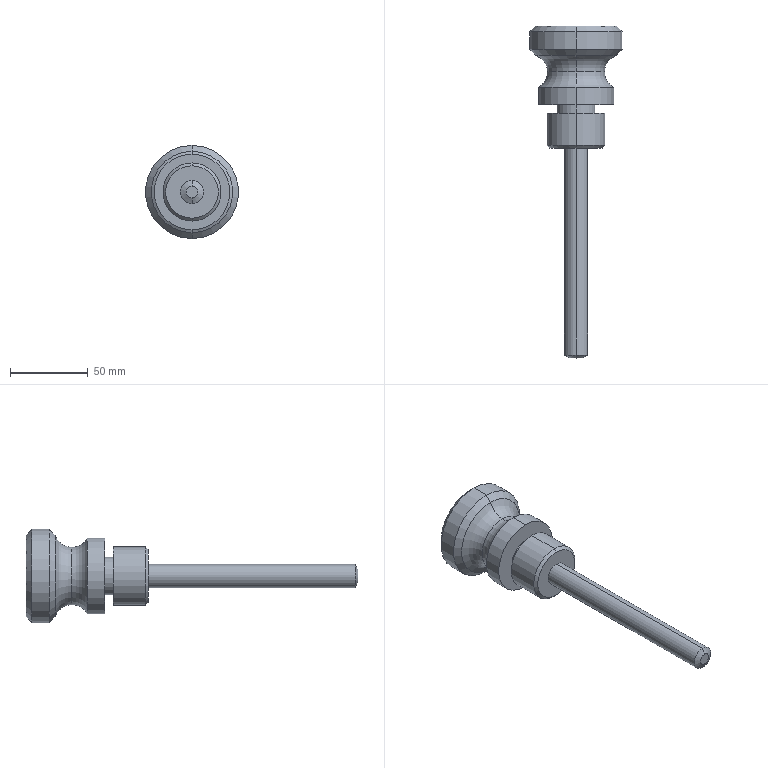Part | SolidWorks | features Revolution 1, Scale 1 | 1 solid | 27 faces | box 60 x 213.75 x 60 mm | volume 149521 mm3 | cylinder 10 | cone 8 | plane 5 | torus 4 | commonest cylinder face diameters 15 x2 24.375 x2 37.5 x2 48.75 x2 60 x2
STEP:
#1=CARTESIAN_POINT('',(0.,6.534,26.25));
#2=VERTEX_POINT('',#1);
#3=CARTESIAN_POINT('',(0.,-4.176,18.442));
#4=VERTEX_POINT('',#3);
#5=CARTESIAN_POINT('',(0.,-4.176,29.692));
#6=DIRECTION('',(-1.,0.,0.));
#7=DIRECTION('',(0.,0.,1.));
#8=AXIS2_PLACEMENT_3D('',#5,#6,#7);
#9=CIRCLE('',#8,11.25);
#10=EDGE_CURVE('',#2,#4,#9,.T.);
#11=ORIENTED_EDGE('',*,*,#10,.T.);
#12=CARTESIAN_POINT('',(0.,-4.176,-18.442));
#13=VERTEX_POINT('',#12);
#14=CARTESIAN_POINT('',(0.,-4.176,0.));
#15=DIRECTION('',(0.,1.,0.));
#16=DIRECTION('',(0.,0.,1.));
#17=AXIS2_PLACEMENT_3D('',#14,#15,#16);
#18=CIRCLE('',#17,18.442);
#19=EDGE_CURVE('',#4,#13,#18,.T.);
#20=ORIENTED_EDGE('',*,*,#19,.T.);
#21=CARTESIAN_POINT('',(0.,6.534,-26.25));
#22=VERTEX_POINT('',#21);
#23=CARTESIAN_POINT('',(0.,-4.176,-29.692));
#24=DIRECTION('',(1.,0.,0.));
#25=DIRECTION('',(0.,0.,-1.));
#26=AXIS2_PLACEMENT_3D('',#23,#24,#25);
#27=CIRCLE('',#26,11.25);
#28=EDGE_CURVE('',#22,#13,#27,.T.);
#29=ORIENTED_EDGE('',*,*,#28,.F.);
#30=CARTESIAN_POINT('',(0.,6.534,0.));
#31=DIRECTION('',(0.,1.,0.));
#32=DIRECTION('',(0.,0.,1.));
#33=AXIS2_PLACEMENT_3D('',#30,#31,#32);
#34=CIRCLE('',#33,26.25);
#35=EDGE_CURVE('',#2,#22,#34,.T.);
#36=ORIENTED_EDGE('',*,*,#35,.F.);
#37=EDGE_LOOP('',(#11,#20,#29,#36));
#38=FACE_OUTER_BOUND('',#37,.T.);
#39=CARTESIAN_POINT('',(0.,-4.176,0.));
#40=DIRECTION('',(0.,1.,0.));
#41=DIRECTION('',(0.,0.,1.));
#42=AXIS2_PLACEMENT_3D('',#39,#40,#41);
#43=TOROIDAL_SURFACE('',#42,29.692,11.25);
#44=ADVANCED_FACE('',(#38),#43,.F.);
#45=ORIENTED_EDGE('',*,*,#28,.T.);
#46=CARTESIAN_POINT('',(0.,-4.176,0.));
#47=DIRECTION('',(0.,1.,0.));
#48=DIRECTION('',(0.,0.,1.));
#49=AXIS2_PLACEMENT_3D('',#46,#47,#48);
#50=CIRCLE('',#49,18.442);
#51=EDGE_CURVE('',#13,#4,#50,.T.);
#52=ORIENTED_EDGE('',*,*,#51,.T.);
#53=ORIENTED_EDGE('',*,*,#10,.F.);
#54=CARTESIAN_POINT('',(0.,6.534,0.));
#55=DIRECTION('',(0.,1.,0.));
#56=DIRECTION('',(0.,0.,1.));
#57=AXIS2_PLACEMENT_3D('',#54,#55,#56);
#58=CIRCLE('',#57,26.25);
#59=EDGE_CURVE('',#22,#2,#58,.T.);
#60=ORIENTED_EDGE('',*,*,#59,.F.);
#61=EDGE_LOOP('',(#45,#52,#53,#60));
#62=FACE_OUTER_BOUND('',#61,.T.);
#63=CARTESIAN_POINT('',(0.,-4.176,0.));
#64=DIRECTION('',(0.,1.,0.));
#65=DIRECTION('',(0.,0.,1.));
#66=AXIS2_PLACEMENT_3D('',#63,#64,#65);
#67=TOROIDAL_SURFACE('',#66,29.692,11.25);
#68=ADVANCED_FACE('',(#62),#67,.F.);
#69=CARTESIAN_POINT('',(0.,-186.591,7.5));
#70=VERTEX_POINT('',#69);
#71=CARTESIAN_POINT('',(0.,-186.591,-7.5));
#72=VERTEX_POINT('',#71);
#73=CARTESIAN_POINT('',(0.,-186.591,0.));
#74=DIRECTION('',(0.,1.,0.));
#75=DIRECTION('',(0.,0.,1.));
#76=AXIS2_PLACEMENT_3D('',#73,#74,#75);
#77=CIRCLE('',#76,7.5);
#78=EDGE_CURVE('',#70,#72,#77,.T.);
#79=ORIENTED_EDGE('',*,*,#78,.T.);
#80=CARTESIAN_POINT('',(0.,-53.466,-7.5));
#81=VERTEX_POINT('',#80);
#82=CARTESIAN_POINT('',(0.,25.284,-7.5));
#83=DIRECTION('',(0.,1.,0.));
#84=VECTOR('',#83,1000.);
#85=LINE('',#82,#84);
#86=EDGE_CURVE('',#72,#81,#85,.T.);
#87=ORIENTED_EDGE('',*,*,#86,.T.);
#88=CARTESIAN_POINT('',(0.,-53.466,7.5));
#89=VERTEX_POINT('',#88);
#90=CARTESIAN_POINT('',(0.,-53.466,0.));
#91=DIRECTION('',(0.,1.,0.));
#92=DIRECTION('',(0.,0.,1.));
#93=AXIS2_PLACEMENT_3D('',#90,#91,#92);
#94=CIRCLE('',#93,7.5);
#95=EDGE_CURVE('',#89,#81,#94,.T.);
#96=ORIENTED_EDGE('',*,*,#95,.F.);
#97=CARTESIAN_POINT('',(0.,25.284,7.5));
#98=DIRECTION('',(0.,1.,0.));
#99=VECTOR('',#98,1000.);
#100=LINE('',#97,#99);
#101=EDGE_CURVE('',#70,#89,#100,.T.);
#102=ORIENTED_EDGE('',*,*,#101,.F.);
#103=EDGE_LOOP('',(#79,#87,#96,#102));
#104=FACE_OUTER_BOUND('',#103,.T.);
#105=CARTESIAN_POINT('',(0.,25.284,0.));
#106=DIRECTION('',(0.,1.,0.));
#107=DIRECTION('',(0.,0.,1.));
#108=AXIS2_PLACEMENT_3D('',#105,#106,#107);
#109=CYLINDRICAL_SURFACE('',#108,7.5);
#110=ADVANCED_FACE('',(#104),#109,.T.);
#111=CARTESIAN_POINT('',(0.,-188.466,3.75));
#112=VERTEX_POINT('',#111);
#113=CARTESIAN_POINT('',(0.,-188.466,-3.75));
#114=VERTEX_POINT('',#113);
#115=CARTESIAN_POINT('',(0.,-188.466,0.));
#116=DIRECTION('',(0.,1.,0.));
#117=DIRECTION('',(0.,0.,1.));
#118=AXIS2_PLACEMENT_3D('',#115,#116,#117);
#119=CIRCLE('',#118,3.75);
#120=EDGE_CURVE('',#112,#114,#119,.T.);
#121=ORIENTED_EDGE('',*,*,#120,.T.);
#122=CARTESIAN_POINT('',(0.,-188.466,-3.75));
#123=DIRECTION('',(0.,0.4472,-0.8944));
#124=VECTOR('',#123,1000.);
#125=LINE('',#122,#124);
#126=EDGE_CURVE('',#114,#72,#125,.T.);
#127=ORIENTED_EDGE('',*,*,#126,.T.);
#128=ORIENTED_EDGE('',*,*,#78,.F.);
#129=CARTESIAN_POINT('',(0.,-188.466,3.75));
#130=DIRECTION('',(0.,0.4472,0.8944));
#131=VECTOR('',#130,1000.);
#132=LINE('',#129,#131);
#133=EDGE_CURVE('',#112,#70,#132,.T.);
#134=ORIENTED_EDGE('',*,*,#133,.F.);
#135=EDGE_LOOP('',(#121,#127,#128,#134));
#136=FACE_OUTER_BOUND('',#135,.T.);
#137=CARTESIAN_POINT('',(0.,-188.466,0.));
#138=DIRECTION('',(0.,1.,0.));
#139=DIRECTION('',(0.,0.,1.));
#140=AXIS2_PLACEMENT_3D('',#137,#138,#139);
#141=CONICAL_SURFACE('',#140,3.75,1.107);
#142=ADVANCED_FACE('',(#136),#141,.T.);
#143=CARTESIAN_POINT('',(0.,25.284,26.25));
#144=VERTEX_POINT('',#143);
#145=CARTESIAN_POINT('',(0.,25.284,-26.25));
#146=VERTEX_POINT('',#145);
#147=CARTESIAN_POINT('',(0.,25.284,0.));
#148=DIRECTION('',(0.,1.,0.));
#149=DIRECTION('',(0.,0.,1.));
#150=AXIS2_PLACEMENT_3D('',#147,#148,#149);
#151=CIRCLE('',#150,26.25);
#152=EDGE_CURVE('',#144,#146,#151,.T.);
#153=ORIENTED_EDGE('',*,*,#152,.F.);
#154=CARTESIAN_POINT('',(0.,21.534,30.));
#155=VERTEX_POINT('',#154);
#156=CARTESIAN_POINT('',(0.,21.534,30.));
#157=DIRECTION('',(0.,-0.7071,0.7071));
#158=VECTOR('',#157,1000.);
#159=LINE('',#156,#158);
#160=EDGE_CURVE('',#144,#155,#159,.T.);
#161=ORIENTED_EDGE('',*,*,#160,.T.);
#162=CARTESIAN_POINT('',(0.,21.534,-30.));
#163=VERTEX_POINT('',#162);
#164=CARTESIAN_POINT('',(0.,21.534,0.));
#165=DIRECTION('',(0.,1.,0.));
#166=DIRECTION('',(0.,0.,1.));
#167=AXIS2_PLACEMENT_3D('',#164,#165,#166);
#168=CIRCLE('',#167,30.);
#169=EDGE_CURVE('',#155,#163,#168,.T.);
#170=ORIENTED_EDGE('',*,*,#169,.T.);
#171=CARTESIAN_POINT('',(0.,21.534,-30.));
#172=DIRECTION('',(0.,-0.7071,-0.7071));
#173=VECTOR('',#172,1000.);
#174=LINE('',#171,#173);
#175=EDGE_CURVE('',#146,#163,#174,.T.);
#176=ORIENTED_EDGE('',*,*,#175,.F.);
#177=EDGE_LOOP('',(#153,#161,#170,#176));
#178=FACE_OUTER_BOUND('',#177,.T.);
#179=CARTESIAN_POINT('',(0.,21.534,0.));
#180=DIRECTION('',(0.,-1.,0.));
#181=DIRECTION('',(0.,0.,-1.));
#182=AXIS2_PLACEMENT_3D('',#179,#180,#181);
#183=CONICAL_SURFACE('',#182,30.,0.7854);
#184=ADVANCED_FACE('',(#178),#183,.T.);
#185=CARTESIAN_POINT('',(0.,10.284,30.));
#186=VERTEX_POINT('',#185);
#187=CARTESIAN_POINT('',(0.,10.284,-30.));
#188=VERTEX_POINT('',#187);
#189=CARTESIAN_POINT('',(0.,10.284,0.));
#190=DIRECTION('',(0.,1.,0.));
#191=DIRECTION('',(0.,0.,1.));
#192=AXIS2_PLACEMENT_3D('',#189,#190,#191);
#193=CIRCLE('',#192,30.);
#194=EDGE_CURVE('',#186,#188,#193,.T.);
#195=ORIENTED_EDGE('',*,*,#194,.T.);
#196=CARTESIAN_POINT('',(0.,25.284,-30.));
#197=DIRECTION('',(0.,1.,0.));
#198=VECTOR('',#197,1000.);
#199=LINE('',#196,#198);
#200=EDGE_CURVE('',#188,#163,#199,.T.);
#201=ORIENTED_EDGE('',*,*,#200,.T.);
#202=ORIENTED_EDGE('',*,*,#169,.F.);
#203=CARTESIAN_POINT('',(0.,25.284,30.));
#204=DIRECTION('',(0.,1.,0.));
#205=VECTOR('',#204,1000.);
#206=LINE('',#203,#205);
#207=EDGE_CURVE('',#186,#155,#206,.T.);
#208=ORIENTED_EDGE('',*,*,#207,.F.);
#209=EDGE_LOOP('',(#195,#201,#202,#208));
#210=FACE_OUTER_BOUND('',#209,.T.);
#211=CARTESIAN_POINT('',(0.,25.284,0.));
#212=DIRECTION('',(0.,1.,0.));
#213=DIRECTION('',(0.,0.,1.));
#214=AXIS2_PLACEMENT_3D('',#211,#212,#213);
#215=CYLINDRICAL_SURFACE('',#214,30.);
#216=ADVANCED_FACE('',(#210),#215,.T.);
#217=ORIENTED_EDGE('',*,*,#35,.T.);
#218=CARTESIAN_POINT('',(0.,6.534,-26.25));
#219=DIRECTION('',(0.,0.7071,-0.7071));
#220=VECTOR('',#219,1000.);
#221=LINE('',#218,#220);
#222=EDGE_CURVE('',#22,#188,#221,.T.);
#223=ORIENTED_EDGE('',*,*,#222,.T.);
#224=ORIENTED_EDGE('',*,*,#194,.F.);
#225=CARTESIAN_POINT('',(0.,6.534,26.25));
#226=DIRECTION('',(0.,0.7071,0.7071));
#227=VECTOR('',#226,1000.);
#228=LINE('',#225,#227);
#229=EDGE_CURVE('',#2,#186,#228,.T.);
#230=ORIENTED_EDGE('',*,*,#229,.F.);
#231=EDGE_LOOP('',(#217,#223,#224,#230));
#232=FACE_OUTER_BOUND('',#231,.T.);
#233=CARTESIAN_POINT('',(0.,6.534,0.));
#234=DIRECTION('',(0.,1.,0.));
#235=DIRECTION('',(0.,0.,1.));
#236=AXIS2_PLACEMENT_3D('',#233,#234,#235);
#237=CONICAL_SURFACE('',#236,26.25,0.7854);
#238=ADVANCED_FACE('',(#232),#237,.T.);
#239=ORIENTED_EDGE('',*,*,#51,.F.);
#240=CARTESIAN_POINT('',(0.,-14.091,-24.375));
#241=VERTEX_POINT('',#240);
#242=CARTESIAN_POINT('',(0.,-4.176,-29.692));
#243=DIRECTION('',(1.,0.,0.));
#244=DIRECTION('',(0.,0.,-1.));
#245=AXIS2_PLACEMENT_3D('',#242,#243,#244);
#246=CIRCLE('',#245,11.25);
#247=EDGE_CURVE('',#13,#241,#246,.T.);
#248=ORIENTED_EDGE('',*,*,#247,.T.);
#249=CARTESIAN_POINT('',(0.,-14.091,24.375));
#250=VERTEX_POINT('',#249);
#251=CARTESIAN_POINT('',(0.,-14.091,0.));
#252=DIRECTION('',(0.,1.,0.));
#253=DIRECTION('',(0.,0.,1.));
#254=AXIS2_PLACEMENT_3D('',#251,#252,#253);
#255=CIRCLE('',#254,24.375);
#256=EDGE_CURVE('',#241,#250,#255,.T.);
#257=ORIENTED_EDGE('',*,*,#256,.T.);
#258=CARTESIAN_POINT('',(0.,-4.176,29.692));
#259=DIRECTION('',(-1.,0.,0.));
#260=DIRECTION('',(0.,0.,1.));
#261=AXIS2_PLACEMENT_3D('',#258,#259,#260);
#262=CIRCLE('',#261,11.25);
#263=EDGE_CURVE('',#4,#250,#262,.T.);
#264=ORIENTED_EDGE('',*,*,#263,.F.);
#265=EDGE_LOOP('',(#239,#248,#257,#264));
#266=FACE_OUTER_BOUND('',#265,.T.);
#267=CARTESIAN_POINT('',(0.,-4.176,0.));
#268=DIRECTION('',(0.,1.,0.));
#269=DIRECTION('',(0.,0.,1.));
#270=AXIS2_PLACEMENT_3D('',#267,#268,#269);
#271=TOROIDAL_SURFACE('',#270,29.692,11.25);
#272=ADVANCED_FACE('',(#266),#271,.F.);
#273=CARTESIAN_POINT('',(0.,-25.341,24.375));
#274=VERTEX_POINT('',#273);
#275=CARTESIAN_POINT('',(0.,-25.341,-24.375));
#276=VERTEX_POINT('',#275);
#277=CARTESIAN_POINT('',(0.,-25.341,0.));
#278=DIRECTION('',(0.,1.,0.));
#279=DIRECTION('',(0.,0.,1.));
#280=AXIS2_PLACEMENT_3D('',#277,#278,#279);
#281=CIRCLE('',#280,24.375);
#282=EDGE_CURVE('',#274,#276,#281,.T.);
#283=ORIENTED_EDGE('',*,*,#282,.T.);
#284=CARTESIAN_POINT('',(0.,25.284,-24.375));
#285=DIRECTION('',(0.,1.,0.));
#286=VECTOR('',#285,1000.);
#287=LINE('',#284,#286);
#288=EDGE_CURVE('',#276,#241,#287,.T.);
#289=ORIENTED_EDGE('',*,*,#288,.T.);
#290=CARTESIAN_POINT('',(0.,-14.091,0.));
#291=DIRECTION('',(0.,1.,0.));
#292=DIRECTION('',(0.,0.,1.));
#293=AXIS2_PLACEMENT_3D('',#290,#291,#292);
#294=CIRCLE('',#293,24.375);
#295=EDGE_CURVE('',#250,#241,#294,.T.);
#296=ORIENTED_EDGE('',*,*,#295,.F.);
#297=CARTESIAN_POINT('',(0.,25.284,24.375));
#298=DIRECTION('',(0.,1.,0.));
#299=VECTOR('',#298,1000.);
#300=LINE('',#297,#299);
#301=EDGE_CURVE('',#274,#250,#300,.T.);
#302=ORIENTED_EDGE('',*,*,#301,.F.);
#303=EDGE_LOOP('',(#283,#289,#296,#302));
#304=FACE_OUTER_BOUND('',#303,.T.);
#305=CARTESIAN_POINT('',(0.,25.284,0.));
#306=DIRECTION('',(0.,1.,0.));
#307=DIRECTION('',(0.,0.,1.));
#308=AXIS2_PLACEMENT_3D('',#305,#306,#307);
#309=CYLINDRICAL_SURFACE('',#308,24.375);
#310=ADVANCED_FACE('',(#304),#309,.T.);
#311=CARTESIAN_POINT('',(0.,-30.966,12.187));
#312=VERTEX_POINT('',#311);
#313=CARTESIAN_POINT('',(0.,-30.966,-12.188));
#314=VERTEX_POINT('',#313);
#315=CARTESIAN_POINT('',(0.,-30.966,0.));
#316=DIRECTION('',(0.,1.,0.));
#317=DIRECTION('',(0.,0.,1.));
#318=AXIS2_PLACEMENT_3D('',#315,#316,#317);
#319=CIRCLE('',#318,12.187);
#320=EDGE_CURVE('',#312,#314,#319,.T.);
#321=ORIENTED_EDGE('',*,*,#320,.T.);
#322=CARTESIAN_POINT('',(0.,-25.341,-12.187));
#323=VERTEX_POINT('',#322);
#324=CARTESIAN_POINT('',(0.,25.284,-12.187));
#325=DIRECTION('',(0.,1.,0.));
#326=VECTOR('',#325,1000.);
#327=LINE('',#324,#326);
#328=EDGE_CURVE('',#314,#323,#327,.T.);
#329=ORIENTED_EDGE('',*,*,#328,.T.);
#330=CARTESIAN_POINT('',(0.,-25.341,12.187));
#331=VERTEX_POINT('',#330);
#332=CARTESIAN_POINT('',(0.,-25.341,0.));
#333=DIRECTION('',(0.,1.,0.));
#334=DIRECTION('',(0.,0.,1.));
#335=AXIS2_PLACEMENT_3D('',#332,#333,#334);
#336=CIRCLE('',#335,12.187);
#337=EDGE_CURVE('',#331,#323,#336,.T.);
#338=ORIENTED_EDGE('',*,*,#337,.F.);
#339=CARTESIAN_POINT('',(0.,25.284,12.187));
#340=DIRECTION('',(0.,1.,0.));
#341=VECTOR('',#340,1000.);
#342=LINE('',#339,#341);
#343=EDGE_CURVE('',#312,#331,#342,.T.);
#344=ORIENTED_EDGE('',*,*,#343,.F.);
#345=EDGE_LOOP('',(#321,#329,#338,#344));
#346=FACE_OUTER_BOUND('',#345,.T.);
#347=CARTESIAN_POINT('',(0.,25.284,0.));
#348=DIRECTION('',(0.,1.,0.));
#349=DIRECTION('',(0.,0.,1.));
#350=AXIS2_PLACEMENT_3D('',#347,#348,#349);
#351=CYLINDRICAL_SURFACE('',#350,12.187);
#352=ADVANCED_FACE('',(#346),#351,.T.);
#353=CARTESIAN_POINT('',(0.,-51.591,18.75));
#354=VERTEX_POINT('',#353);
#355=CARTESIAN_POINT('',(0.,-51.591,-18.75));
#356=VERTEX_POINT('',#355);
#357=CARTESIAN_POINT('',(0.,-51.591,0.));
#358=DIRECTION('',(0.,1.,0.));
#359=DIRECTION('',(0.,0.,1.));
#360=AXIS2_PLACEMENT_3D('',#357,#358,#359);
#361=CIRCLE('',#360,18.75);
#362=EDGE_CURVE('',#354,#356,#361,.T.);
#363=ORIENTED_EDGE('',*,*,#362,.T.);
#364=CARTESIAN_POINT('',(0.,-30.966,-18.75));
#365=VERTEX_POINT('',#364);
#366=CARTESIAN_POINT('',(0.,25.284,-18.75));
#367=DIRECTION('',(0.,1.,0.));
#368=VECTOR('',#367,1000.);
#369=LINE('',#366,#368);
#370=EDGE_CURVE('',#356,#365,#369,.T.);
#371=ORIENTED_EDGE('',*,*,#370,.T.);
#372=CARTESIAN_POINT('',(0.,-30.966,18.75));
#373=VERTEX_POINT('',#372);
#374=CARTESIAN_POINT('',(0.,-30.966,0.));
#375=DIRECTION('',(0.,1.,0.));
#376=DIRECTION('',(0.,0.,1.));
#377=AXIS2_PLACEMENT_3D('',#374,#375,#376);
#378=CIRCLE('',#377,18.75);
#379=EDGE_CURVE('',#373,#365,#378,.T.);
#380=ORIENTED_EDGE('',*,*,#379,.F.);
#381=CARTESIAN_POINT('',(0.,25.284,18.75));
#382=DIRECTION('',(0.,1.,0.));
#383=VECTOR('',#382,1000.);
#384=LINE('',#381,#383);
#385=EDGE_CURVE('',#354,#373,#384,.T.);
#386=ORIENTED_EDGE('',*,*,#385,.F.);
#387=EDGE_LOOP('',(#363,#371,#380,#386));
#388=FACE_OUTER_BOUND('',#387,.T.);
#389=CARTESIAN_POINT('',(0.,25.284,0.));
#390=DIRECTION('',(0.,1.,0.));
#391=DIRECTION('',(0.,0.,1.));
#392=AXIS2_PLACEMENT_3D('',#389,#390,#391);
#393=CYLINDRICAL_SURFACE('',#392,18.75);
#394=ADVANCED_FACE('',(#388),#393,.T.);
#395=CARTESIAN_POINT('',(0.,-53.466,16.875));
#396=VERTEX_POINT('',#395);
#397=CARTESIAN_POINT('',(0.,-53.466,-16.875));
#398=VERTEX_POINT('',#397);
#399=CARTESIAN_POINT('',(0.,-53.466,0.));
#400=DIRECTION('',(0.,1.,0.));
#401=DIRECTION('',(0.,0.,1.));
#402=AXIS2_PLACEMENT_3D('',#399,#400,#401);
#403=CIRCLE('',#402,16.875);
#404=EDGE_CURVE('',#396,#398,#403,.T.);
#405=ORIENTED_EDGE('',*,*,#404,.T.);
#406=CARTESIAN_POINT('',(0.,-53.466,-16.875));
#407=DIRECTION('',(0.,0.7071,-0.7071));
#408=VECTOR('',#407,1000.);
#409=LINE('',#406,#408);
#410=EDGE_CURVE('',#398,#356,#409,.T.);
#411=ORIENTED_EDGE('',*,*,#410,.T.);
#412=ORIENTED_EDGE('',*,*,#362,.F.);
#413=CARTESIAN_POINT('',(0.,-53.466,16.875));
#414=DIRECTION('',(0.,0.7071,0.7071));
#415=VECTOR('',#414,1000.);
#416=LINE('',#413,#415);
#417=EDGE_CURVE('',#396,#354,#416,.T.);
#418=ORIENTED_EDGE('',*,*,#417,.F.);
#419=EDGE_LOOP('',(#405,#411,#412,#418));
#420=FACE_OUTER_BOUND('',#419,.T.);
#421=CARTESIAN_POINT('',(0.,-53.466,0.));
#422=DIRECTION('',(0.,1.,0.));
#423=DIRECTION('',(0.,0.,1.));
#424=AXIS2_PLACEMENT_3D('',#421,#422,#423);
#425=CONICAL_SURFACE('',#424,16.875,0.7854);
#426=ADVANCED_FACE('',(#420),#425,.T.);
#427=ORIENTED_EDGE('',*,*,#404,.F.);
#428=CARTESIAN_POINT('',(0.,-53.466,0.));
#429=DIRECTION('',(0.,1.,0.));
#430=DIRECTION('',(0.,0.,1.));
#431=AXIS2_PLACEMENT_3D('',#428,#429,#430);
#432=CIRCLE('',#431,16.875);
#433=EDGE_CURVE('',#398,#396,#432,.T.);
#434=ORIENTED_EDGE('',*,*,#433,.F.);
#435=EDGE_LOOP('',(#427,#434));
#436=FACE_OUTER_BOUND('',#435,.T.);
#437=ORIENTED_EDGE('',*,*,#95,.T.);
#438=CARTESIAN_POINT('',(0.,-53.466,0.));
#439=DIRECTION('',(0.,1.,0.));
#440=DIRECTION('',(0.,0.,1.));
#441=AXIS2_PLACEMENT_3D('',#438,#439,#440);
#442=CIRCLE('',#441,7.5);
#443=EDGE_CURVE('',#81,#89,#442,.T.);
#444=ORIENTED_EDGE('',*,*,#443,.T.);
#445=EDGE_LOOP('',(#437,#444));
#446=FACE_BOUND('',#445,.T.);
#447=CARTESIAN_POINT('',(7.5,-53.466,0.));
#448=DIRECTION('',(0.,1.,0.));
#449=DIRECTION('',(0.,0.,1.));
#450=AXIS2_PLACEMENT_3D('',#447,#448,#449);
#451=PLANE('',#450);
#452=ADVANCED_FACE('',(#436,#446),#451,.F.);
#453=ORIENTED_EDGE('',*,*,#410,.F.);
#454=ORIENTED_EDGE('',*,*,#433,.T.);
#455=ORIENTED_EDGE('',*,*,#417,.T.);
#456=CARTESIAN_POINT('',(0.,-51.591,0.));
#457=DIRECTION('',(0.,1.,0.));
#458=DIRECTION('',(0.,0.,1.));
#459=AXIS2_PLACEMENT_3D('',#456,#457,#458);
#460=CIRCLE('',#459,18.75);
#461=EDGE_CURVE('',#356,#354,#460,.T.);
#462=ORIENTED_EDGE('',*,*,#461,.F.);
#463=EDGE_LOOP('',(#453,#454,#455,#462));
#464=FACE_OUTER_BOUND('',#463,.T.);
#465=CARTESIAN_POINT('',(0.,-53.466,0.));
#466=DIRECTION('',(0.,1.,0.));
#467=DIRECTION('',(0.,0.,1.));
#468=AXIS2_PLACEMENT_3D('',#465,#466,#467);
#469=CONICAL_SURFACE('',#468,16.875,0.7854);
#470=ADVANCED_FACE('',(#464),#469,.T.);
#471=ORIENTED_EDGE('',*,*,#370,.F.);
#472=ORIENTED_EDGE('',*,*,#461,.T.);
#473=ORIENTED_EDGE('',*,*,#385,.T.);
#474=CARTESIAN_POINT('',(0.,-30.966,0.));
#475=DIRECTION('',(0.,1.,0.));
#476=DIRECTION('',(0.,0.,1.));
#477=AXIS2_PLACEMENT_3D('',#474,#475,#476);
#478=CIRCLE('',#477,18.75);
#479=EDGE_CURVE('',#365,#373,#478,.T.);
#480=ORIENTED_EDGE('',*,*,#479,.F.);
#481=EDGE_LOOP('',(#471,#472,#473,#480));
#482=FACE_OUTER_BOUND('',#481,.T.);
#483=CARTESIAN_POINT('',(0.,25.284,0.));
#484=DIRECTION('',(0.,1.,0.));
#485=DIRECTION('',(0.,0.,1.));
#486=AXIS2_PLACEMENT_3D('',#483,#484,#485);
#487=CYLINDRICAL_SURFACE('',#486,18.75);
#488=ADVANCED_FACE('',(#482),#487,.T.);
#489=ORIENTED_EDGE('',*,*,#320,.F.);
#490=CARTESIAN_POINT('',(0.,-30.966,0.));
#491=DIRECTION('',(0.,1.,0.));
#492=DIRECTION('',(0.,0.,1.));
#493=AXIS2_PLACEMENT_3D('',#490,#491,#492);
#494=CIRCLE('',#493,12.187);
#495=EDGE_CURVE('',#314,#312,#494,.T.);
#496=ORIENTED_EDGE('',*,*,#495,.F.);
#497=EDGE_LOOP('',(#489,#496));
#498=FACE_BOUND('',#497,.T.);
#499=ORIENTED_EDGE('',*,*,#379,.T.);
#500=ORIENTED_EDGE('',*,*,#479,.T.);
#501=EDGE_LOOP('',(#499,#500));
#502=FACE_OUTER_BOUND('',#501,.T.);
#503=CARTESIAN_POINT('',(12.187,-30.966,0.));
#504=DIRECTION('',(0.,-1.,0.));
#505=DIRECTION('',(0.,0.,-1.));
#506=AXIS2_PLACEMENT_3D('',#503,#504,#505);
#507=PLANE('',#506);
#508=ADVANCED_FACE('',(#498,#502),#507,.F.);
#509=ORIENTED_EDGE('',*,*,#328,.F.);
#510=ORIENTED_EDGE('',*,*,#495,.T.);
#511=ORIENTED_EDGE('',*,*,#343,.T.);
#512=CARTESIAN_POINT('',(0.,-25.341,0.));
#513=DIRECTION('',(0.,1.,0.));
#514=DIRECTION('',(0.,0.,1.));
#515=AXIS2_PLACEMENT_3D('',#512,#513,#514);
#516=CIRCLE('',#515,12.187);
#517=EDGE_CURVE('',#323,#331,#516,.T.);
#518=ORIENTED_EDGE('',*,*,#517,.F.);
#519=EDGE_LOOP('',(#509,#510,#511,#518));
#520=FACE_OUTER_BOUND('',#519,.T.);
#521=CARTESIAN_POINT('',(0.,25.284,0.));
#522=DIRECTION('',(0.,1.,0.));
#523=DIRECTION('',(0.,0.,1.));
#524=AXIS2_PLACEMENT_3D('',#521,#522,#523);
#525=CYLINDRICAL_SURFACE('',#524,12.187);
#526=ADVANCED_FACE('',(#520),#525,.T.);
#527=ORIENTED_EDGE('',*,*,#282,.F.);
#528=CARTESIAN_POINT('',(0.,-25.341,0.));
#529=DIRECTION('',(0.,1.,0.));
#530=DIRECTION('',(0.,0.,1.));
#531=AXIS2_PLACEMENT_3D('',#528,#529,#530);
#532=CIRCLE('',#531,24.375);
#533=EDGE_CURVE('',#276,#274,#532,.T.);
#534=ORIENTED_EDGE('',*,*,#533,.F.);
#535=EDGE_LOOP('',(#527,#534));
#536=FACE_OUTER_BOUND('',#535,.T.);
#537=ORIENTED_EDGE('',*,*,#337,.T.);
#538=ORIENTED_EDGE('',*,*,#517,.T.);
#539=EDGE_LOOP('',(#537,#538));
#540=FACE_BOUND('',#539,.T.);
#541=CARTESIAN_POINT('',(24.375,-25.341,0.));
#542=DIRECTION('',(0.,1.,0.));
#543=DIRECTION('',(0.,0.,1.));
#544=AXIS2_PLACEMENT_3D('',#541,#542,#543);
#545=PLANE('',#544);
#546=ADVANCED_FACE('',(#536,#540),#545,.F.);
#547=ORIENTED_EDGE('',*,*,#288,.F.);
#548=ORIENTED_EDGE('',*,*,#533,.T.);
#549=ORIENTED_EDGE('',*,*,#301,.T.);
#550=ORIENTED_EDGE('',*,*,#256,.F.);
#551=EDGE_LOOP('',(#547,#548,#549,#550));
#552=FACE_OUTER_BOUND('',#551,.T.);
#553=CARTESIAN_POINT('',(0.,25.284,0.));
#554=DIRECTION('',(0.,1.,0.));
#555=DIRECTION('',(0.,0.,1.));
#556=AXIS2_PLACEMENT_3D('',#553,#554,#555);
#557=CYLINDRICAL_SURFACE('',#556,24.375);
#558=ADVANCED_FACE('',(#552),#557,.T.);
#559=ORIENTED_EDGE('',*,*,#19,.F.);
#560=ORIENTED_EDGE('',*,*,#263,.T.);
#561=ORIENTED_EDGE('',*,*,#295,.T.);
#562=ORIENTED_EDGE('',*,*,#247,.F.);
#563=EDGE_LOOP('',(#559,#560,#561,#562));
#564=FACE_OUTER_BOUND('',#563,.T.);
#565=CARTESIAN_POINT('',(0.,-4.176,0.));
#566=DIRECTION('',(0.,1.,0.));
#567=DIRECTION('',(0.,0.,1.));
#568=AXIS2_PLACEMENT_3D('',#565,#566,#567);
#569=TOROIDAL_SURFACE('',#568,29.692,11.25);
#570=ADVANCED_FACE('',(#564),#569,.F.);
#571=ORIENTED_EDGE('',*,*,#222,.F.);
#572=ORIENTED_EDGE('',*,*,#59,.T.);
#573=ORIENTED_EDGE('',*,*,#229,.T.);
#574=CARTESIAN_POINT('',(0.,10.284,0.));
#575=DIRECTION('',(0.,1.,0.));
#576=DIRECTION('',(0.,0.,1.));
#577=AXIS2_PLACEMENT_3D('',#574,#575,#576);
#578=CIRCLE('',#577,30.);
#579=EDGE_CURVE('',#188,#186,#578,.T.);
#580=ORIENTED_EDGE('',*,*,#579,.F.);
#581=EDGE_LOOP('',(#571,#572,#573,#580));
#582=FACE_OUTER_BOUND('',#581,.T.);
#583=CARTESIAN_POINT('',(0.,6.534,0.));
#584=DIRECTION('',(0.,1.,0.));
#585=DIRECTION('',(0.,0.,1.));
#586=AXIS2_PLACEMENT_3D('',#583,#584,#585);
#587=CONICAL_SURFACE('',#586,26.25,0.7854);
#588=ADVANCED_FACE('',(#582),#587,.T.);
#589=ORIENTED_EDGE('',*,*,#200,.F.);
#590=ORIENTED_EDGE('',*,*,#579,.T.);
#591=ORIENTED_EDGE('',*,*,#207,.T.);
#592=CARTESIAN_POINT('',(0.,21.534,0.));
#593=DIRECTION('',(0.,1.,0.));
#594=DIRECTION('',(0.,0.,1.));
#595=AXIS2_PLACEMENT_3D('',#592,#593,#594);
#596=CIRCLE('',#595,30.);
#597=EDGE_CURVE('',#163,#155,#596,.T.);
#598=ORIENTED_EDGE('',*,*,#597,.F.);
#599=EDGE_LOOP('',(#589,#590,#591,#598));
#600=FACE_OUTER_BOUND('',#599,.T.);
#601=CARTESIAN_POINT('',(0.,25.284,0.));
#602=DIRECTION('',(0.,1.,0.));
#603=DIRECTION('',(0.,0.,1.));
#604=AXIS2_PLACEMENT_3D('',#601,#602,#603);
#605=CYLINDRICAL_SURFACE('',#604,30.);
#606=ADVANCED_FACE('',(#600),#605,.T.);
#607=ORIENTED_EDGE('',*,*,#160,.F.);
#608=CARTESIAN_POINT('',(0.,25.284,0.));
#609=DIRECTION('',(0.,1.,0.));
#610=DIRECTION('',(0.,0.,1.));
#611=AXIS2_PLACEMENT_3D('',#608,#609,#610);
#612=CIRCLE('',#611,26.25);
#613=EDGE_CURVE('',#146,#144,#612,.T.);
#614=ORIENTED_EDGE('',*,*,#613,.F.);
#615=ORIENTED_EDGE('',*,*,#175,.T.);
#616=ORIENTED_EDGE('',*,*,#597,.T.);
#617=EDGE_LOOP('',(#607,#614,#615,#616));
#618=FACE_OUTER_BOUND('',#617,.T.);
#619=CARTESIAN_POINT('',(0.,21.534,0.));
#620=DIRECTION('',(0.,-1.,0.));
#621=DIRECTION('',(0.,0.,-1.));
#622=AXIS2_PLACEMENT_3D('',#619,#620,#621);
#623=CONICAL_SURFACE('',#622,30.,0.7854);
#624=ADVANCED_FACE('',(#618),#623,.T.);
#625=ORIENTED_EDGE('',*,*,#613,.T.);
#626=ORIENTED_EDGE('',*,*,#152,.T.);
#627=EDGE_LOOP('',(#625,#626));
#628=FACE_OUTER_BOUND('',#627,.T.);
#629=CARTESIAN_POINT('',(0.,25.284,0.));
#630=DIRECTION('',(0.,-1.,0.));
#631=DIRECTION('',(0.,0.,-1.));
#632=AXIS2_PLACEMENT_3D('',#629,#630,#631);
#633=PLANE('',#632);
#634=ADVANCED_FACE('',(#628),#633,.F.);
#635=ORIENTED_EDGE('',*,*,#120,.F.);
#636=CARTESIAN_POINT('',(0.,-188.466,0.));
#637=DIRECTION('',(0.,1.,0.));
#638=DIRECTION('',(0.,0.,1.));
#639=AXIS2_PLACEMENT_3D('',#636,#637,#638);
#640=CIRCLE('',#639,3.75);
#641=EDGE_CURVE('',#114,#112,#640,.T.);
#642=ORIENTED_EDGE('',*,*,#641,.F.);
#643=EDGE_LOOP('',(#635,#642));
#644=FACE_OUTER_BOUND('',#643,.T.);
#645=CARTESIAN_POINT('',(0.,-188.466,0.));
#646=DIRECTION('',(0.,1.,0.));
#647=DIRECTION('',(0.,0.,1.));
#648=AXIS2_PLACEMENT_3D('',#645,#646,#647);
#649=PLANE('',#648);
#650=ADVANCED_FACE('',(#644),#649,.F.);
#651=ORIENTED_EDGE('',*,*,#126,.F.);
#652=ORIENTED_EDGE('',*,*,#641,.T.);
#653=ORIENTED_EDGE('',*,*,#133,.T.);
#654=CARTESIAN_POINT('',(0.,-186.591,0.));
#655=DIRECTION('',(0.,1.,0.));
#656=DIRECTION('',(0.,0.,1.));
#657=AXIS2_PLACEMENT_3D('',#654,#655,#656);
#658=CIRCLE('',#657,7.5);
#659=EDGE_CURVE('',#72,#70,#658,.T.);
#660=ORIENTED_EDGE('',*,*,#659,.F.);
#661=EDGE_LOOP('',(#651,#652,#653,#660));
#662=FACE_OUTER_BOUND('',#661,.T.);
#663=CARTESIAN_POINT('',(0.,-188.466,0.));
#664=DIRECTION('',(0.,1.,0.));
#665=DIRECTION('',(0.,0.,1.));
#666=AXIS2_PLACEMENT_3D('',#663,#664,#665);
#667=CONICAL_SURFACE('',#666,3.75,1.107);
#668=ADVANCED_FACE('',(#662),#667,.T.);
#669=ORIENTED_EDGE('',*,*,#86,.F.);
#670=ORIENTED_EDGE('',*,*,#659,.T.);
#671=ORIENTED_EDGE('',*,*,#101,.T.);
#672=ORIENTED_EDGE('',*,*,#443,.F.);
#673=EDGE_LOOP('',(#669,#670,#671,#672));
#674=FACE_OUTER_BOUND('',#673,.T.);
#675=CARTESIAN_POINT('',(0.,25.284,0.));
#676=DIRECTION('',(0.,1.,0.));
#677=DIRECTION('',(0.,0.,1.));
#678=AXIS2_PLACEMENT_3D('',#675,#676,#677);
#679=CYLINDRICAL_SURFACE('',#678,7.5);
#680=ADVANCED_FACE('',(#674),#679,.T.);
#681=CLOSED_SHELL('',(#44,#68,#110,#142,#184,#216,#238,#272,#310,#352,#394,#426,#452,#470,#488,#508,#526,#546,#558,#570,#588,#606,#624,#634,#650,#668,#680));
#682=MANIFOLD_SOLID_BREP('',#681);
#683=CARTESIAN_POINT('',(0.,0.,0.));
#684=DIRECTION('',(0.,0.,1.));
#685=DIRECTION('',(1.,0.,0.));
#686=AXIS2_PLACEMENT_3D('',#683,#684,#685);
#687=(LENGTH_UNIT()NAMED_UNIT(*)SI_UNIT(.MILLI.,.METRE.));
#688=UNCERTAINTY_MEASURE_WITH_UNIT(LENGTH_MEASURE(0.00001),#687,'','');
#689=(NAMED_UNIT(*)PLANE_ANGLE_UNIT()SI_UNIT($,.RADIAN.));
#690=(NAMED_UNIT(*)SI_UNIT($,.STERADIAN.)SOLID_ANGLE_UNIT());
#691=(GEOMETRIC_REPRESENTATION_CONTEXT(3)GLOBAL_UNCERTAINTY_ASSIGNED_CONTEXT((#688))GLOBAL_UNIT_ASSIGNED_CONTEXT((#687,#689,#690))REPRESENTATION_CONTEXT('',''));
#692=ADVANCED_BREP_SHAPE_REPRESENTATION('',(#682,#686),#691);